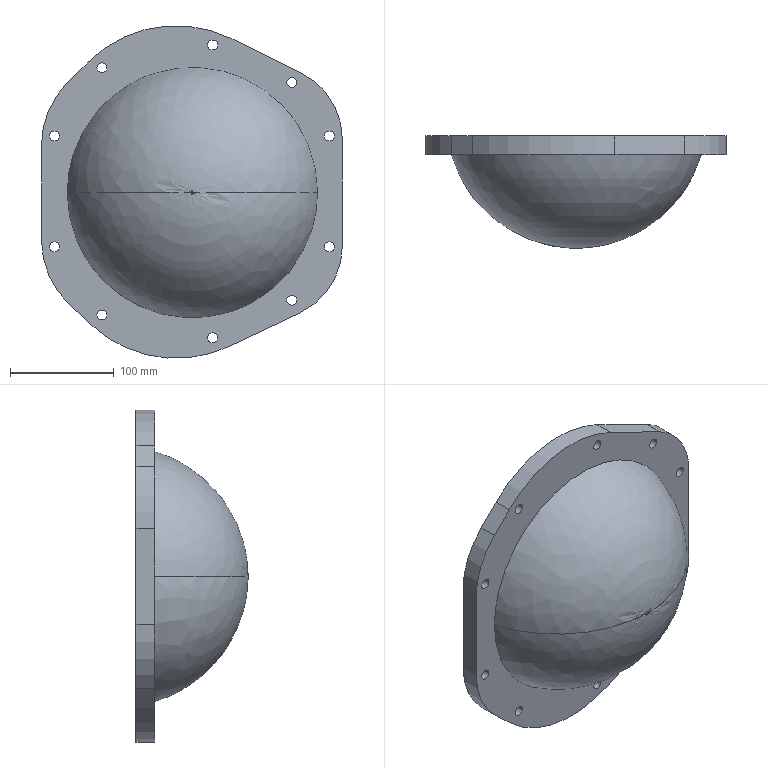Part | NX | features BREP 1 | 1 solid | 42 faces | box 289.8 x 108 x 320.4 mm | volume 1771319 mm3 | cylinder 28 | plane 10 | spline 4 | commonest cylinder face diameters 9.6 x20 144 x2 168 x2 206.564 x2 240 x2